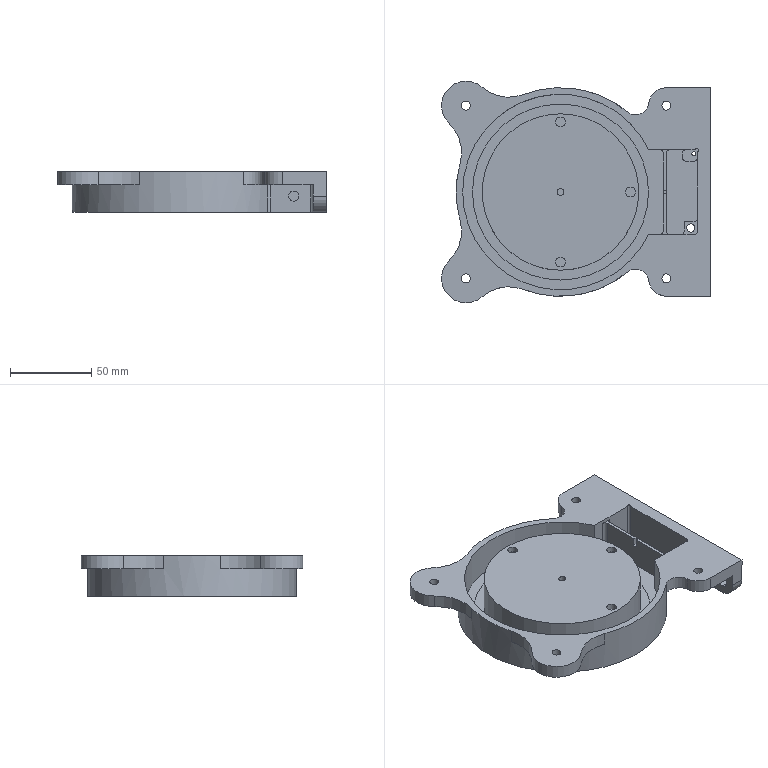NC program | NX | posted with a generic post | part box 165 x 136 x 25 mm
Lines 12422 to 12613 of 16615:
(FLOOR_WALL_1 , TOOL : D10JING)
N24812 T09 M6
N24814 G54
N24816 G17 G0 G90 X-43.55 Y13.987 S9500 M3
N24818 G43 Z30. H9
N24820 Z-20.
N24822 G94 G1 Z-21. F1250.
N24824 G3 X-43. Y14.629 R1.
N24826 G2 X-42.749 Y15.5 R54.5
N24828 G1 X-41.791 Y15.216
N24830 G2 X24.716 Y51.291 R53.5
N24832 X-41.791 Y15.216 R-53.5
N24834 G1 X-42.749 Y15.5
N24836 X-43.
N24838 Y14.629
N24840 X-48.
N24842 Y-14.629
N24844 X-43.
N24846 Y-15.5
N24848 X-42.749
N24850 G2 X-43. Y-14.629 R54.5
N24852 G1 X-48.
N24854 Y-20.5
N24856 X-41.43
N24858 G2 X-40.98 Y-20.783 R0.5
N24860 G1 X-39.617 Y-23.617
N24862 G3 X-39.617 Y23.617 R-54.5
N24864 G1 X-40.98 Y20.783
N24866 G2 X-41.43 Y20.5 R0.5
N24868 G1 X-48.
N24870 Y14.629
N24872 X-48.143 Y15.395
N24874 G3 X-48.5 Y14.629 R1.
N24876 G1 Y-21.
N24878 X-41.43
N24880 X-40.068 Y-23.833
N24882 G3 X-40.068 Y23.833 R-55.
N24884 G1 X-41.43 Y21.
N24886 X-48.5
N24888 Y14.629
N24890 G3 X-48.143 Y13.863 R1.
N24892 G1 X-42.424 Y12.306
N24894 G3 X-41.891 Y12.962 R1.
N24896 G2 X22.462 Y51.391 R53.
N24898 X-41.891 Y12.962 R-53.
N24900 G3 X-42.05 Y13.792 R1.
N24902 G1 X-42.903 Y14.973
N24904 Z-20.
N24906 G0 Z30.
N24908 X-61.766 Y-20.143
N24910 Z-20.
N24912 G1 Z-21.
N24914 G3 X-61. Y-20.5 R1.
N24916 G1 Y20.5
N24918 Y13.
N24920 G2 X-61.5 Y12.5 R0.5
N24922 G1 X-69.
N24924 Y-20.5
N24926 X-61.
N24928 X-61.766 Y-20.643
N24930 G3 X-61. Y-21. R1.
N24932 G1 X-60.5
N24934 Y21.
N24936 X-61.5
N24938 Y13.
N24940 X-69.5
N24942 Y-21.
N24944 X-61.
N24946 G3 X-60.617 Y-20.821 R0.5
N24948 G1 X-61.5 Y-20.
N24950 Z-20.
N24952 G0 Z30.
N24954 Y20.
N24956 Z-1.
N24958 G1 Z-2.
N24960 X-54.734 Y20.143
N24962 G3 X-55.5 Y20.5 R1.
N24964 G1 Y-20.5
N24966 X-53.5
N24968 Y20.5
N24970 X-55.5
N24972 G3 X-56.266 Y20.143 R1.
N24974 G1 X-61.5 Y20.
N24976 Z-1.
N24978 G0 Z1.1
N24980 G1 X-54.5 Y19.5 F8000.
N24982 G0 Z-1.
N24984 G1 Z-2. F1250.
N24986 X-52.734 Y20.643
N24988 G3 X-53.5 Y21. R1.
N24990 G1 X-55.5
N24992 G3 X-56.266 Y20.643 R1.
N24994 G1 X-54.5 Y19.5
N24996 Z-1.
N24998 G0 Z1.1
N25000 G1 Y-19.5 F8000.
N25002 G0 Z-1.
N25004 G1 Z-2. F1250.
N25006 X-56.266 Y-20.643
N25008 G3 X-55.5 Y-21. R1.
N25010 G1 X-53.5
N25012 G3 X-52.734 Y-20.643 R1.
N25014 G1 X-54.5 Y-19.5
N25016 Z-1.
N25018 G0 Z30.
N25020 X-62.141 Y13.876
N25022 Z-19.3
N25024 G1 Z-20.3
N25026 X-66.143 Y17.234
N25028 G2 X-66.5 Y18. R1.
N25030 G1 Y20.5
N25032 X-69.
N25034 Y18.
N25036 X-66.5
N25038 G2 X-65.734 Y17.643 R1.
N25040 G1 X-62.376 Y13.641
N25042 Z-19.3
N25044 G0 Z-17.2
N25046 G1 X-67.5 Y19.5 F8000.
N25048 G0 Z-19.3
N25050 G1 Z-20.3 F1250.
N25052 X-65.734 Y20.643
N25054 G3 X-66.5 Y21. R1.
N25056 G1 X-69.5
N25058 Y18.
N25060 G3 X-69.143 Y17.234 R1.
N25062 G1 X-68. Y19.
N25064 Z-19.3
N25066 G0 Z30.
(ZLEVEL_PROFILE , TOOL : D10JING)
N25068 X-89.463 Y-65.624
N25070 Z-24.
N25072 G1 Z-25.
N25074 X-88.15 Y-64.866
N25076 G3 X-87.65 Y-64. R1.
N25078 G1 Y64.
N25080 G2 X-82.5 Y69.15 R5.15
N25082 G1 X-55.5
N25084 G2 X-39.466 Y54.934 R16.15
N25086 G3 X-34.811 Y53.088 R2.85
N25088 G2 X34.145 Y64.609 R69.15
N25090 G3 X54.261 Y68.191 R19.85
N25092 G2 X81.439 Y38.449 R20.15
N25094 G3 X76.063 Y18.737 R19.85
N25096 G2 X76.063 Y-18.737 R69.15
N25098 G3 X81.439 Y-38.449 R19.85
N25100 G2 X54.261 Y-68.191 R20.15
N25102 G3 X34.145 Y-64.609 R19.85
N25104 G2 X-34.811 Y-53.088 R69.15
N25106 G3 X-39.466 Y-54.934 R2.85
N25108 G2 X-55.5 Y-69.15 R16.15
N25110 G1 X-82.5
N25112 G2 X-87.65 Y-64. R5.15
N25114 G3 X-88.15 Y-63.134 R1.
N25116 G1 X-89.65 Y-62.268
N25118 Z-24.
N25120 G0 Z30.
(ZLEVEL_PROFILE_COPY , TOOL : D10JING)
N25122 X-89.309 Y-65.622
N25124 Z-24.
N25126 G1 Z-25.
N25128 X-88. Y-64.866
N25130 G3 X-87.5 Y-64. R1.
N25132 G1 Y64.
N25134 G2 X-82.5 Y69. R5.
N25136 G1 X-55.5
N25138 G2 X-39.615 Y54.916 R16.
N25140 G3 X-34.714 Y52.973 R3.
N25142 G2 X34.092 Y64.469 R69.
N25144 G3 X54.36 Y68.078 R20.
N25146 G2 X81.335 Y38.558 R20.
N25148 G3 X75.919 Y18.696 R20.
N25150 G2 X75.919 Y-18.696 R69.
N25152 G3 X81.335 Y-38.558 R20.
N25154 G2 X54.36 Y-68.078 R20.
N25156 G3 X34.092 Y-64.469 R20.
N25158 G2 X-34.714 Y-52.973 R69.
N25160 G3 X-39.615 Y-54.916 R3.
N25162 G2 X-55.5 Y-69. R16.
N25164 G1 X-82.5
N25166 G2 X-87.5 Y-64. R5.
N25168 G3 X-88. Y-63.134 R1.
N25170 G1 X-89.5 Y-62.268
N25172 Z-24.
N25174 G0 Z30.
N25176 M5